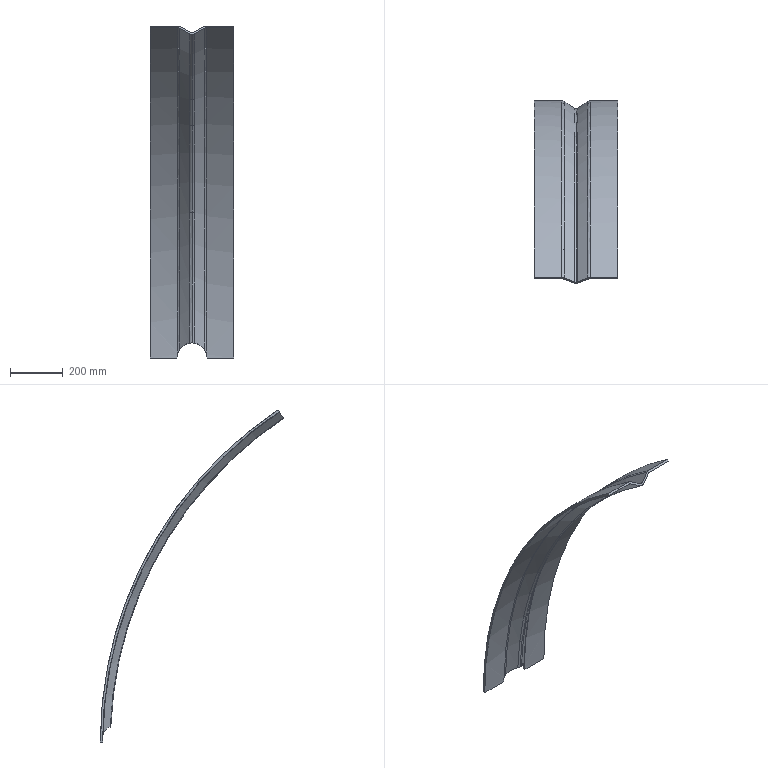Part | SolidWorks | features ICE 1, Sweep 1 | 1 solid | 23 faces | box 317.5 x 695.606 x 1261 mm | volume 3914320 mm3 | torus 8 | cylinder 6 | plane 5 | cone 4 | commonest cylinder face diameters 114.3 x2 3016 x2 3032 x2
STEP:
#1=CARTESIAN_POINT('',(-5.241,-669.592,1237.163));
#2=VERTEX_POINT('',#1);
#3=CARTESIAN_POINT('',(0.,-670.464,1235.856));
#4=VERTEX_POINT('',#3);
#5=CARTESIAN_POINT('',(0.,-665.176,1243.778));
#6=DIRECTION('',(0.,-0.8317,0.5552));
#7=DIRECTION('',(1.,0.,0.));
#8=AXIS2_PLACEMENT_3D('',#5,#6,#7);
#9=CIRCLE('',#8,9.525);
#10=EDGE_CURVE('',#2,#4,#9,.T.);
#11=ORIENTED_EDGE('',*,*,#10,.T.);
#12=CARTESIAN_POINT('',(0.,-10.624,57.15));
#13=VERTEX_POINT('',#12);
#14=CARTESIAN_POINT('',(0.,-1495.425,0.));
#15=DIRECTION('',(-1.,0.,0.));
#16=DIRECTION('',(0.,0.,1.));
#17=AXIS2_PLACEMENT_3D('',#14,#15,#16);
#18=CIRCLE('',#17,1485.9);
#19=EDGE_CURVE('',#4,#13,#18,.T.);
#20=ORIENTED_EDGE('',*,*,#19,.T.);
#21=CARTESIAN_POINT('',(-5.241,-9.042,56.909));
#22=VERTEX_POINT('',#21);
#23=CARTESIAN_POINT('',(-5.241,-9.042,56.909));
#24=CARTESIAN_POINT('',(-4.464,-9.558,56.981));
#25=CARTESIAN_POINT('',(-3.63,-9.95,57.042));
#26=CARTESIAN_POINT('',(-2.518,-10.286,57.095));
#27=CARTESIAN_POINT('',(-2.291,-10.346,57.105));
#28=CARTESIAN_POINT('',(-1.837,-10.447,57.121));
#29=CARTESIAN_POINT('',(-1.609,-10.489,57.128));
#30=CARTESIAN_POINT('',(-0.9231,-10.591,57.144));
#31=CARTESIAN_POINT('',(-0.463,-10.624,57.15));
#32=CARTESIAN_POINT('',(0.,-10.624,57.15));
#33=B_SPLINE_CURVE_WITH_KNOTS('',3,(#23,#24,#25,#26,#27,#28,#29,#30,#31,#32),.UNSPECIFIED.,.F.,.F.,(4,2,2,2,4),(0.000000237,0.002769,0.003461,0.004154,0.005538),.UNSPECIFIED.);
#34=EDGE_CURVE('',#22,#13,#33,.T.);
#35=ORIENTED_EDGE('',*,*,#34,.F.);
#36=CARTESIAN_POINT('',(-5.241,-1495.425,0.));
#37=DIRECTION('',(-1.,0.,0.));
#38=DIRECTION('',(0.,0.,1.));
#39=AXIS2_PLACEMENT_3D('',#36,#37,#38);
#40=CIRCLE('',#39,1487.472);
#41=EDGE_CURVE('',#2,#22,#40,.T.);
#42=ORIENTED_EDGE('',*,*,#41,.F.);
#43=EDGE_LOOP('',(#11,#20,#35,#42));
#44=FACE_OUTER_BOUND('',#43,.T.);
#45=CARTESIAN_POINT('',(0.,-1495.425,0.));
#46=DIRECTION('',(-1.,0.,0.));
#47=DIRECTION('',(0.,0.,1.));
#48=AXIS2_PLACEMENT_3D('',#45,#46,#47);
#49=TOROIDAL_SURFACE('',#48,1495.425,9.525);
#50=ADVANCED_FACE('',(#44),#49,.F.);
#51=CARTESIAN_POINT('',(0.,-674.906,1229.202));
#52=VERTEX_POINT('',#51);
#53=CARTESIAN_POINT('',(9.644,-673.3,1231.607));
#54=VERTEX_POINT('',#53);
#55=CARTESIAN_POINT('',(0.,-665.176,1243.778));
#56=DIRECTION('',(0.,-0.8317,0.5552));
#57=DIRECTION('',(1.,0.,0.));
#58=AXIS2_PLACEMENT_3D('',#55,#56,#57);
#59=CIRCLE('',#58,17.525);
#60=EDGE_CURVE('',#52,#54,#59,.T.);
#61=ORIENTED_EDGE('',*,*,#60,.F.);
#62=CARTESIAN_POINT('',(0.,-18.63,57.15));
#63=VERTEX_POINT('',#62);
#64=CARTESIAN_POINT('',(0.,-1495.425,0.));
#65=DIRECTION('',(-1.,0.,0.));
#66=DIRECTION('',(0.,0.,1.));
#67=AXIS2_PLACEMENT_3D('',#64,#65,#66);
#68=CIRCLE('',#67,1477.9);
#69=EDGE_CURVE('',#52,#63,#68,.T.);
#70=ORIENTED_EDGE('',*,*,#69,.T.);
#71=CARTESIAN_POINT('',(9.644,-15.705,56.33));
#72=VERTEX_POINT('',#71);
#73=CARTESIAN_POINT('',(0.,-18.63,57.15));
#74=CARTESIAN_POINT('',(0.8525,-18.63,57.15));
#75=CARTESIAN_POINT('',(1.717,-18.566,57.13));
#76=CARTESIAN_POINT('',(3.403,-18.314,57.055));
#77=CARTESIAN_POINT('',(4.229,-18.127,56.999));
#78=CARTESIAN_POINT('',(5.447,-17.757,56.891));
#79=CARTESIAN_POINT('',(5.848,-17.619,56.851));
#80=CARTESIAN_POINT('',(6.644,-17.312,56.764));
#81=CARTESIAN_POINT('',(7.038,-17.143,56.716));
#82=CARTESIAN_POINT('',(8.194,-16.596,56.565));
#83=CARTESIAN_POINT('',(8.934,-16.177,56.452));
#84=CARTESIAN_POINT('',(9.644,-15.705,56.33));
#85=B_SPLINE_CURVE_WITH_KNOTS('',3,(#73,#74,#75,#76,#77,#78,#79,#80,#81,#82,#83,#84),.UNSPECIFIED.,.F.,.F.,(4,2,2,2,2,4),(0.01023,0.01277,0.01532,0.0166,0.01787,0.02042),.UNSPECIFIED.);
#86=EDGE_CURVE('',#63,#72,#85,.T.);
#87=ORIENTED_EDGE('',*,*,#86,.T.);
#88=CARTESIAN_POINT('',(9.644,-1495.425,0.));
#89=DIRECTION('',(-1.,0.,0.));
#90=DIRECTION('',(0.,0.,1.));
#91=AXIS2_PLACEMENT_3D('',#88,#89,#90);
#92=CIRCLE('',#91,1480.792);
#93=EDGE_CURVE('',#54,#72,#92,.T.);
#94=ORIENTED_EDGE('',*,*,#93,.F.);
#95=EDGE_LOOP('',(#61,#70,#87,#94));
#96=FACE_OUTER_BOUND('',#95,.T.);
#97=CARTESIAN_POINT('',(0.,-1495.425,0.));
#98=DIRECTION('',(-1.,0.,0.));
#99=DIRECTION('',(0.,0.,1.));
#100=AXIS2_PLACEMENT_3D('',#97,#98,#99);
#101=TOROIDAL_SURFACE('',#100,1495.425,17.525);
#102=ADVANCED_FACE('',(#96),#101,.T.);
#103=ORIENTED_EDGE('',*,*,#86,.F.);
#104=CARTESIAN_POINT('',(0.,-50.,57.15));
#105=DIRECTION('',(0.,1.,0.));
#106=VECTOR('',#105,1000.);
#107=LINE('',#104,#106);
#108=EDGE_CURVE('',#63,#13,#107,.T.);
#109=ORIENTED_EDGE('',*,*,#108,.T.);
#110=CARTESIAN_POINT('',(5.241,-9.042,56.909));
#111=VERTEX_POINT('',#110);
#112=CARTESIAN_POINT('',(0.,-10.624,57.15));
#113=CARTESIAN_POINT('',(0.4615,-10.624,57.15));
#114=CARTESIAN_POINT('',(0.9295,-10.59,57.144));
#115=CARTESIAN_POINT('',(1.845,-10.454,57.122));
#116=CARTESIAN_POINT('',(2.293,-10.354,57.106));
#117=CARTESIAN_POINT('',(3.174,-10.088,57.063));
#118=CARTESIAN_POINT('',(3.608,-9.922,57.038));
#119=CARTESIAN_POINT('',(4.449,-9.527,56.978));
#120=CARTESIAN_POINT('',(4.854,-9.299,56.945));
#121=CARTESIAN_POINT('',(5.241,-9.042,56.909));
#122=B_SPLINE_CURVE_WITH_KNOTS('',3,(#112,#113,#114,#115,#116,#117,#118,#119,#120,#121),.UNSPECIFIED.,.F.,.F.,(4,2,2,2,4),(0.005538,0.006918,0.008298,0.009678,0.01106),.UNSPECIFIED.);
#123=EDGE_CURVE('',#13,#111,#122,.T.);
#124=ORIENTED_EDGE('',*,*,#123,.T.);
#125=CARTESIAN_POINT('',(44.331,17.378,36.067));
#126=VERTEX_POINT('',#125);
#127=CARTESIAN_POINT('',(44.331,17.378,36.067));
#128=CARTESIAN_POINT('',(43.066,16.507,37.622));
#129=CARTESIAN_POINT('',(41.737,15.593,39.09));
#130=CARTESIAN_POINT('',(38.954,13.684,41.864));
#131=CARTESIAN_POINT('',(37.501,12.69,43.169));
#132=CARTESIAN_POINT('',(35.232,11.139,45.008));
#133=CARTESIAN_POINT('',(34.459,10.612,45.603));
#134=CARTESIAN_POINT('',(32.898,9.548,46.741));
#135=CARTESIAN_POINT('',(32.109,9.01,47.287));
#136=CARTESIAN_POINT('',(29.714,7.382,48.855));
#137=CARTESIAN_POINT('',(28.084,6.275,49.809));
#138=CARTESIAN_POINT('',(24.756,4.022,51.544));
#139=CARTESIAN_POINT('',(23.059,2.876,52.325));
#140=CARTESIAN_POINT('',(20.465,1.128,53.368));
#141=CARTESIAN_POINT('',(19.592,0.5412,53.695));
#142=CARTESIAN_POINT('',(17.83,-0.6428,54.305));
#143=CARTESIAN_POINT('',(16.944,-1.238,54.588));
#144=CARTESIAN_POINT('',(12.499,-4.217,55.889));
#145=CARTESIAN_POINT('',(8.895,-6.62,56.573));
#146=CARTESIAN_POINT('',(5.241,-9.042,56.909));
#147=B_SPLINE_CURVE_WITH_KNOTS('',3,(#127,#128,#129,#130,#131,#132,#133,#134,#135,#136,#137,#138,#139,#140,#141,#142,#143,#144,#145,#146),.UNSPECIFIED.,.F.,.F.,(4,2,2,2,2,2,2,2,2,4),(0.007159,0.0137,0.02025,0.02352,0.0268,0.03334,0.03989,0.04316,0.04643,0.05952),.UNSPECIFIED.);
#148=EDGE_CURVE('',#126,#111,#147,.T.);
#149=ORIENTED_EDGE('',*,*,#148,.F.);
#150=CARTESIAN_POINT('',(53.975,20.584,18.784));
#151=VERTEX_POINT('',#150);
#152=CARTESIAN_POINT('',(44.331,17.378,36.067));
#153=CARTESIAN_POINT('',(45.318,18.058,34.854));
#154=CARTESIAN_POINT('',(46.28,18.58,33.57));
#155=CARTESIAN_POINT('',(47.661,19.202,31.547));
#156=CARTESIAN_POINT('',(48.112,19.382,30.856));
#157=CARTESIAN_POINT('',(48.989,19.696,29.442));
#158=CARTESIAN_POINT('',(49.418,19.83,28.718));
#159=CARTESIAN_POINT('',(50.65,20.171,26.523));
#160=CARTESIAN_POINT('',(51.408,20.319,25.023));
#161=CARTESIAN_POINT('',(52.791,20.516,21.955));
#162=CARTESIAN_POINT('',(53.417,20.564,20.386));
#163=CARTESIAN_POINT('',(53.975,20.584,18.784));
#164=B_SPLINE_CURVE_WITH_KNOTS('',3,(#152,#153,#154,#155,#156,#157,#158,#159,#160,#161,#162,#163),.UNSPECIFIED.,.F.,.F.,(4,2,2,2,2,4),(0.000000341,0.005054,0.007581,0.01011,0.01516,0.02022),.UNSPECIFIED.);
#165=EDGE_CURVE('',#126,#151,#164,.T.);
#166=ORIENTED_EDGE('',*,*,#165,.T.);
#167=CARTESIAN_POINT('',(57.15,20.7,0.));
#168=VERTEX_POINT('',#167);
#169=CARTESIAN_POINT('',(57.15,20.7,0.));
#170=CARTESIAN_POINT('',(57.15,20.7,3.22));
#171=CARTESIAN_POINT('',(56.88,20.69,6.395));
#172=CARTESIAN_POINT('',(55.821,20.65,12.656));
#173=CARTESIAN_POINT('',(55.033,20.621,15.743));
#174=CARTESIAN_POINT('',(53.975,20.584,18.784));
#175=B_SPLINE_CURVE_WITH_KNOTS('',3,(#169,#170,#171,#172,#173,#174),.UNSPECIFIED.,.F.,.F.,(4,2,4),(0.,0.009525,0.01905),.UNSPECIFIED.);
#176=EDGE_CURVE('',#168,#151,#175,.T.);
#177=ORIENTED_EDGE('',*,*,#176,.F.);
#178=CARTESIAN_POINT('',(57.15,12.7,0.));
#179=VERTEX_POINT('',#178);
#180=CARTESIAN_POINT('',(57.15,-50.,0.));
#181=DIRECTION('',(0.,1.,0.));
#182=VECTOR('',#181,1000.);
#183=LINE('',#180,#182);
#184=EDGE_CURVE('',#179,#168,#183,.T.);
#185=ORIENTED_EDGE('',*,*,#184,.F.);
#186=CARTESIAN_POINT('',(53.975,12.583,18.784));
#187=VERTEX_POINT('',#186);
#188=CARTESIAN_POINT('',(57.15,12.7,0.));
#189=CARTESIAN_POINT('',(57.15,12.7,3.22));
#190=CARTESIAN_POINT('',(56.88,12.69,6.395));
#191=CARTESIAN_POINT('',(55.821,12.65,12.656));
#192=CARTESIAN_POINT('',(55.033,12.621,15.743));
#193=CARTESIAN_POINT('',(53.975,12.583,18.784));
#194=B_SPLINE_CURVE_WITH_KNOTS('',3,(#188,#189,#190,#191,#192,#193),.UNSPECIFIED.,.F.,.F.,(4,2,4),(0.,0.009525,0.01905),.UNSPECIFIED.);
#195=EDGE_CURVE('',#179,#187,#194,.T.);
#196=ORIENTED_EDGE('',*,*,#195,.T.);
#197=CARTESIAN_POINT('',(48.734,10.832,29.852));
#198=VERTEX_POINT('',#197);
#199=CARTESIAN_POINT('',(48.734,10.832,29.852));
#200=CARTESIAN_POINT('',(49.248,11.188,29.013));
#201=CARTESIAN_POINT('',(49.748,11.464,28.148));
#202=CARTESIAN_POINT('',(50.71,11.908,26.375));
#203=CARTESIAN_POINT('',(51.172,12.075,25.467));
#204=CARTESIAN_POINT('',(52.055,12.331,23.611));
#205=CARTESIAN_POINT('',(52.476,12.42,22.66));
#206=CARTESIAN_POINT('',(53.264,12.539,20.739));
#207=CARTESIAN_POINT('',(53.633,12.571,19.767));
#208=CARTESIAN_POINT('',(53.975,12.583,18.784));
#209=B_SPLINE_CURVE_WITH_KNOTS('',3,(#199,#200,#201,#202,#203,#204,#205,#206,#207,#208),.UNSPECIFIED.,.F.,.F.,(4,2,2,2,4),(0.000000402,0.003097,0.006194,0.009291,0.01239),.UNSPECIFIED.);
#210=EDGE_CURVE('',#198,#187,#209,.T.);
#211=ORIENTED_EDGE('',*,*,#210,.F.);
#212=CARTESIAN_POINT('',(48.734,10.832,29.852));
#213=CARTESIAN_POINT('',(47.603,10.051,31.698));
#214=CARTESIAN_POINT('',(46.381,9.207,33.459));
#215=CARTESIAN_POINT('',(44.417,7.853,35.978));
#216=CARTESIAN_POINT('',(43.74,7.387,36.797));
#217=CARTESIAN_POINT('',(42.344,6.427,38.396));
#218=CARTESIAN_POINT('',(41.625,5.933,39.173));
#219=CARTESIAN_POINT('',(39.431,4.427,41.421));
#220=CARTESIAN_POINT('',(37.91,3.384,42.815));
#221=CARTESIAN_POINT('',(34.757,1.229,45.412));
#222=CARTESIAN_POINT('',(33.126,0.1169,46.614));
#223=CARTESIAN_POINT('',(29.759,-2.174,48.832));
#224=CARTESIAN_POINT('',(28.016,-3.358,49.852));
#225=CARTESIAN_POINT('',(24.486,-5.747,51.677));
#226=CARTESIAN_POINT('',(22.694,-6.958,52.488));
#227=CARTESIAN_POINT('',(19.055,-9.408,53.915));
#228=CARTESIAN_POINT('',(17.21,-10.648,54.532));
#229=CARTESIAN_POINT('',(14.401,-12.529,55.314));
#230=CARTESIAN_POINT('',(13.459,-13.159,55.551));
#231=CARTESIAN_POINT('',(11.56,-14.427,55.977));
#232=CARTESIAN_POINT('',(10.603,-15.066,56.166));
#233=CARTESIAN_POINT('',(9.644,-15.705,56.33));
#234=B_SPLINE_CURVE_WITH_KNOTS('',3,(#212,#213,#214,#215,#216,#217,#218,#219,#220,#221,#222,#223,#224,#225,#226,#227,#228,#229,#230,#231,#232,#233),.UNSPECIFIED.,.F.,.F.,(4,2,2,2,2,2,2,2,2,2,4),(0.008928,0.01583,0.01928,0.02273,0.02964,0.03654,0.04344,0.05035,0.05725,0.0607,0.06415),.UNSPECIFIED.);
#235=EDGE_CURVE('',#198,#72,#234,.T.);
#236=ORIENTED_EDGE('',*,*,#235,.T.);
#237=EDGE_LOOP('',(#103,#109,#124,#149,#166,#177,#185,#196,#211,#236));
#238=FACE_OUTER_BOUND('',#237,.T.);
#239=CARTESIAN_POINT('',(0.,-50.,0.));
#240=DIRECTION('',(0.,1.,0.));
#241=DIRECTION('',(0.,0.,1.));
#242=AXIS2_PLACEMENT_3D('',#239,#240,#241);
#243=CYLINDRICAL_SURFACE('',#242,57.15);
#244=ADVANCED_FACE('',(#238),#243,.F.);
#245=CARTESIAN_POINT('',(158.75,12.7,0.));
#246=VERTEX_POINT('',#245);
#247=CARTESIAN_POINT('',(158.75,12.7,0.));
#248=DIRECTION('',(-1.,0.,0.));
#249=VECTOR('',#248,1000.);
#250=LINE('',#247,#249);
#251=EDGE_CURVE('',#246,#179,#250,.T.);
#252=ORIENTED_EDGE('',*,*,#251,.T.);
#253=ORIENTED_EDGE('',*,*,#184,.T.);
#254=CARTESIAN_POINT('',(158.75,20.7,0.));
#255=VERTEX_POINT('',#254);
#256=CARTESIAN_POINT('',(158.75,20.7,0.));
#257=DIRECTION('',(-1.,0.,0.));
#258=VECTOR('',#257,1000.);
#259=LINE('',#256,#258);
#260=EDGE_CURVE('',#255,#168,#259,.T.);
#261=ORIENTED_EDGE('',*,*,#260,.F.);
#262=CARTESIAN_POINT('',(158.75,20.7,0.));
#263=DIRECTION('',(0.,-1.,0.));
#264=VECTOR('',#263,1000.);
#265=LINE('',#262,#264);
#266=EDGE_CURVE('',#255,#246,#265,.T.);
#267=ORIENTED_EDGE('',*,*,#266,.T.);
#268=EDGE_LOOP('',(#252,#253,#261,#267));
#269=FACE_OUTER_BOUND('',#268,.T.);
#270=CARTESIAN_POINT('',(-53.975,3.175,0.));
#271=DIRECTION('',(0.,0.,1.));
#272=DIRECTION('',(1.,0.,0.));
#273=AXIS2_PLACEMENT_3D('',#270,#271,#272);
#274=PLANE('',#273);
#275=ADVANCED_FACE('',(#269),#274,.F.);
#276=CARTESIAN_POINT('',(-158.75,-658.125,1254.341));
#277=VERTEX_POINT('',#276);
#278=CARTESIAN_POINT('',(-158.75,12.7,0.));
#279=VERTEX_POINT('',#278);
#280=CARTESIAN_POINT('',(-158.75,-1495.425,0.));
#281=DIRECTION('',(-1.,0.,0.));
#282=DIRECTION('',(0.,0.,1.));
#283=AXIS2_PLACEMENT_3D('',#280,#281,#282);
#284=CIRCLE('',#283,1508.125);
#285=EDGE_CURVE('',#277,#279,#284,.T.);
#286=ORIENTED_EDGE('',*,*,#285,.F.);
#287=CARTESIAN_POINT('',(-158.75,-653.684,1260.994));
#288=VERTEX_POINT('',#287);
#289=CARTESIAN_POINT('',(-158.75,-653.684,1260.994));
#290=DIRECTION('',(0.,-0.5552,-0.8317));
#291=VECTOR('',#290,1000.);
#292=LINE('',#289,#291);
#293=EDGE_CURVE('',#288,#277,#292,.T.);
#294=ORIENTED_EDGE('',*,*,#293,.F.);
#295=CARTESIAN_POINT('',(-158.75,20.7,0.));
#296=VERTEX_POINT('',#295);
#297=CARTESIAN_POINT('',(-158.75,-1495.425,0.));
#298=DIRECTION('',(-1.,0.,0.));
#299=DIRECTION('',(0.,0.,1.));
#300=AXIS2_PLACEMENT_3D('',#297,#298,#299);
#301=CIRCLE('',#300,1516.125);
#302=EDGE_CURVE('',#288,#296,#301,.T.);
#303=ORIENTED_EDGE('',*,*,#302,.T.);
#304=CARTESIAN_POINT('',(-158.75,20.7,0.));
#305=DIRECTION('',(0.,-1.,0.));
#306=VECTOR('',#305,1000.);
#307=LINE('',#304,#306);
#308=EDGE_CURVE('',#296,#279,#307,.T.);
#309=ORIENTED_EDGE('',*,*,#308,.T.);
#310=EDGE_LOOP('',(#286,#294,#303,#309));
#311=FACE_OUTER_BOUND('',#310,.T.);
#312=CARTESIAN_POINT('',(-158.75,-653.684,1260.994));
#313=DIRECTION('',(1.,0.,0.));
#314=DIRECTION('',(0.,0.,-1.));
#315=AXIS2_PLACEMENT_3D('',#312,#313,#314);
#316=PLANE('',#315);
#317=ADVANCED_FACE('',(#311),#316,.F.);
#318=CARTESIAN_POINT('',(-57.15,12.7,0.));
#319=VERTEX_POINT('',#318);
#320=CARTESIAN_POINT('',(-158.75,12.7,0.));
#321=DIRECTION('',(1.,0.,0.));
#322=VECTOR('',#321,1000.);
#323=LINE('',#320,#322);
#324=EDGE_CURVE('',#279,#319,#323,.T.);
#325=ORIENTED_EDGE('',*,*,#324,.T.);
#326=CARTESIAN_POINT('',(-53.975,12.583,18.784));
#327=VERTEX_POINT('',#326);
#328=CARTESIAN_POINT('',(-57.15,12.7,0.));
#329=CARTESIAN_POINT('',(-57.15,12.7,3.22));
#330=CARTESIAN_POINT('',(-56.88,12.69,6.395));
#331=CARTESIAN_POINT('',(-55.821,12.65,12.656));
#332=CARTESIAN_POINT('',(-55.033,12.621,15.743));
#333=CARTESIAN_POINT('',(-53.975,12.583,18.784));
#334=B_SPLINE_CURVE_WITH_KNOTS('',3,(#328,#329,#330,#331,#332,#333),.UNSPECIFIED.,.F.,.F.,(4,2,4),(0.,0.009525,0.01905),.UNSPECIFIED.);
#335=EDGE_CURVE('',#319,#327,#334,.T.);
#336=ORIENTED_EDGE('',*,*,#335,.T.);
#337=CARTESIAN_POINT('',(-53.975,-658.125,1254.341));
#338=VERTEX_POINT('',#337);
#339=CARTESIAN_POINT('',(-53.975,-1495.425,0.));
#340=DIRECTION('',(-1.,0.,0.));
#341=DIRECTION('',(0.,0.,1.));
#342=AXIS2_PLACEMENT_3D('',#339,#340,#341);
#343=CIRCLE('',#342,1508.125);
#344=EDGE_CURVE('',#338,#327,#343,.T.);
#345=ORIENTED_EDGE('',*,*,#344,.F.);
#346=CARTESIAN_POINT('',(-158.75,-658.125,1254.341));
#347=DIRECTION('',(1.,0.,0.));
#348=VECTOR('',#347,1000.);
#349=LINE('',#346,#348);
#350=EDGE_CURVE('',#277,#338,#349,.T.);
#351=ORIENTED_EDGE('',*,*,#350,.F.);
#352=ORIENTED_EDGE('',*,*,#285,.T.);
#353=EDGE_LOOP('',(#325,#336,#345,#351,#352));
#354=FACE_OUTER_BOUND('',#353,.T.);
#355=CARTESIAN_POINT('',(0.,-1495.425,0.));
#356=DIRECTION('',(-1.,0.,0.));
#357=DIRECTION('',(0.,0.,1.));
#358=AXIS2_PLACEMENT_3D('',#355,#356,#357);
#359=CYLINDRICAL_SURFACE('',#358,1508.125);
#360=ADVANCED_FACE('',(#354),#359,.F.);
#361=CARTESIAN_POINT('',(-48.734,10.832,29.852));
#362=VERTEX_POINT('',#361);
#363=CARTESIAN_POINT('',(-48.734,10.832,29.852));
#364=CARTESIAN_POINT('',(-49.248,11.188,29.013));
#365=CARTESIAN_POINT('',(-49.748,11.464,28.148));
#366=CARTESIAN_POINT('',(-50.71,11.908,26.375));
#367=CARTESIAN_POINT('',(-51.172,12.075,25.467));
#368=CARTESIAN_POINT('',(-52.055,12.331,23.611));
#369=CARTESIAN_POINT('',(-52.476,12.42,22.66));
#370=CARTESIAN_POINT('',(-53.264,12.539,20.739));
#371=CARTESIAN_POINT('',(-53.633,12.571,19.767));
#372=CARTESIAN_POINT('',(-53.975,12.583,18.784));
#373=B_SPLINE_CURVE_WITH_KNOTS('',3,(#363,#364,#365,#366,#367,#368,#369,#370,#371,#372),.UNSPECIFIED.,.F.,.F.,(4,2,2,2,4),(0.000000402,0.003097,0.006194,0.009291,0.01239),.UNSPECIFIED.);
#374=EDGE_CURVE('',#362,#327,#373,.T.);
#375=ORIENTED_EDGE('',*,*,#374,.F.);
#376=CARTESIAN_POINT('',(-48.734,-658.998,1253.033));
#377=VERTEX_POINT('',#376);
#378=CARTESIAN_POINT('',(-48.734,-1495.425,0.));
#379=DIRECTION('',(-1.,0.,0.));
#380=DIRECTION('',(0.,0.,1.));
#381=AXIS2_PLACEMENT_3D('',#378,#379,#380);
#382=CIRCLE('',#381,1506.553);
#383=EDGE_CURVE('',#377,#362,#382,.T.);
#384=ORIENTED_EDGE('',*,*,#383,.F.);
#385=CARTESIAN_POINT('',(-53.975,-663.413,1246.418));
#386=DIRECTION('',(0.,-0.8317,0.5552));
#387=DIRECTION('',(1.,0.,0.));
#388=AXIS2_PLACEMENT_3D('',#385,#386,#387);
#389=CIRCLE('',#388,9.525);
#390=EDGE_CURVE('',#377,#338,#389,.T.);
#391=ORIENTED_EDGE('',*,*,#390,.T.);
#392=ORIENTED_EDGE('',*,*,#344,.T.);
#393=EDGE_LOOP('',(#375,#384,#391,#392));
#394=FACE_OUTER_BOUND('',#393,.T.);
#395=CARTESIAN_POINT('',(-53.975,-1495.425,0.));
#396=DIRECTION('',(-1.,0.,0.));
#397=DIRECTION('',(0.,0.,1.));
#398=AXIS2_PLACEMENT_3D('',#395,#396,#397);
#399=TOROIDAL_SURFACE('',#398,1498.6,9.525);
#400=ADVANCED_FACE('',(#394),#399,.F.);
#401=ORIENTED_EDGE('',*,*,#383,.T.);
#402=CARTESIAN_POINT('',(-9.644,-15.705,56.33));
#403=VERTEX_POINT('',#402);
#404=CARTESIAN_POINT('',(-48.734,10.832,29.852));
#405=CARTESIAN_POINT('',(-47.603,10.051,31.698));
#406=CARTESIAN_POINT('',(-46.381,9.207,33.459));
#407=CARTESIAN_POINT('',(-44.417,7.853,35.978));
#408=CARTESIAN_POINT('',(-43.74,7.387,36.797));
#409=CARTESIAN_POINT('',(-42.344,6.427,38.396));
#410=CARTESIAN_POINT('',(-41.625,5.933,39.173));
#411=CARTESIAN_POINT('',(-39.431,4.427,41.421));
#412=CARTESIAN_POINT('',(-37.91,3.384,42.815));
#413=CARTESIAN_POINT('',(-34.757,1.229,45.412));
#414=CARTESIAN_POINT('',(-33.126,0.1169,46.614));
#415=CARTESIAN_POINT('',(-29.759,-2.174,48.832));
#416=CARTESIAN_POINT('',(-28.016,-3.358,49.852));
#417=CARTESIAN_POINT('',(-24.486,-5.747,51.677));
#418=CARTESIAN_POINT('',(-22.694,-6.958,52.488));
#419=CARTESIAN_POINT('',(-19.055,-9.408,53.915));
#420=CARTESIAN_POINT('',(-17.21,-10.648,54.532));
#421=CARTESIAN_POINT('',(-14.401,-12.529,55.314));
#422=CARTESIAN_POINT('',(-13.459,-13.159,55.551));
#423=CARTESIAN_POINT('',(-11.56,-14.427,55.977));
#424=CARTESIAN_POINT('',(-10.603,-15.066,56.166));
#425=CARTESIAN_POINT('',(-9.644,-15.705,56.33));
#426=B_SPLINE_CURVE_WITH_KNOTS('',3,(#404,#405,#406,#407,#408,#409,#410,#411,#412,#413,#414,#415,#416,#417,#418,#419,#420,#421,#422,#423,#424,#425),.UNSPECIFIED.,.F.,.F.,(4,2,2,2,2,2,2,2,2,2,4),(0.008928,0.01583,0.01928,0.02273,0.02964,0.03654,0.04344,0.05035,0.05725,0.0607,0.06415),.UNSPECIFIED.);
#427=EDGE_CURVE('',#362,#403,#426,.T.);
#428=ORIENTED_EDGE('',*,*,#427,.T.);
#429=CARTESIAN_POINT('',(-9.644,-673.3,1231.607));
#430=VERTEX_POINT('',#429);
#431=CARTESIAN_POINT('',(-9.644,-1495.425,0.));
#432=DIRECTION('',(-1.,0.,0.));
#433=DIRECTION('',(0.,0.,1.));
#434=AXIS2_PLACEMENT_3D('',#431,#432,#433);
#435=CIRCLE('',#434,1480.792);
#436=EDGE_CURVE('',#430,#403,#435,.T.);
#437=ORIENTED_EDGE('',*,*,#436,.F.);
#438=CARTESIAN_POINT('',(-48.734,-658.998,1253.033));
#439=DIRECTION('',(0.835,-0.3055,-0.4577));
#440=VECTOR('',#439,1000.);
#441=LINE('',#438,#440);
#442=EDGE_CURVE('',#377,#430,#441,.T.);
#443=ORIENTED_EDGE('',*,*,#442,.F.);
#444=EDGE_LOOP('',(#401,#428,#437,#443));
#445=FACE_OUTER_BOUND('',#444,.T.);
#446=CARTESIAN_POINT('',(-48.734,-1495.425,0.));
#447=DIRECTION('',(-1.,0.,0.));
#448=DIRECTION('',(0.,0.,1.));
#449=AXIS2_PLACEMENT_3D('',#446,#447,#448);
#450=CONICAL_SURFACE('',#449,1506.553,0.5827);
#451=ADVANCED_FACE('',(#445),#450,.F.);
#452=ORIENTED_EDGE('',*,*,#69,.F.);
#453=CARTESIAN_POINT('',(0.,-665.176,1243.778));
#454=DIRECTION('',(0.,-0.8317,0.5552));
#455=DIRECTION('',(1.,0.,0.));
#456=AXIS2_PLACEMENT_3D('',#453,#454,#455);
#457=CIRCLE('',#456,17.525);
#458=EDGE_CURVE('',#430,#52,#457,.T.);
#459=ORIENTED_EDGE('',*,*,#458,.F.);
#460=ORIENTED_EDGE('',*,*,#436,.T.);
#461=CARTESIAN_POINT('',(-9.644,-15.705,56.33));
#462=CARTESIAN_POINT('',(-8.932,-16.179,56.452));
#463=CARTESIAN_POINT('',(-8.193,-16.596,56.565));
#464=CARTESIAN_POINT('',(-6.663,-17.321,56.766));
#465=CARTESIAN_POINT('',(-5.872,-17.628,56.854));
#466=CARTESIAN_POINT('',(-4.643,-18.002,56.963));
#467=CARTESIAN_POINT('',(-4.225,-18.113,56.995));
#468=CARTESIAN_POINT('',(-3.388,-18.301,57.051));
#469=CARTESIAN_POINT('',(-2.969,-18.379,57.074));
#470=CARTESIAN_POINT('',(-1.705,-18.567,57.131));
#471=CARTESIAN_POINT('',(-0.8555,-18.63,57.15));
#472=CARTESIAN_POINT('',(0.,-18.63,57.15));
#473=B_SPLINE_CURVE_WITH_KNOTS('',3,(#461,#462,#463,#464,#465,#466,#467,#468,#469,#470,#471,#472),.UNSPECIFIED.,.F.,.F.,(4,2,2,2,2,4),(0.000000239,0.002557,0.005113,0.006392,0.00767,0.01023),.UNSPECIFIED.);
#474=EDGE_CURVE('',#403,#63,#473,.T.);
#475=ORIENTED_EDGE('',*,*,#474,.T.);
#476=EDGE_LOOP('',(#452,#459,#460,#475));
#477=FACE_OUTER_BOUND('',#476,.T.);
#478=CARTESIAN_POINT('',(0.,-1495.425,0.));
#479=DIRECTION('',(-1.,0.,0.));
#480=DIRECTION('',(0.,0.,1.));
#481=AXIS2_PLACEMENT_3D('',#478,#479,#480);
#482=TOROIDAL_SURFACE('',#481,1495.425,17.525);
#483=ADVANCED_FACE('',(#477),#482,.T.);
#484=ORIENTED_EDGE('',*,*,#235,.F.);
#485=CARTESIAN_POINT('',(48.734,-658.998,1253.033));
#486=VERTEX_POINT('',#485);
#487=CARTESIAN_POINT('',(48.734,-1495.425,0.));
#488=DIRECTION('',(-1.,0.,0.));
#489=DIRECTION('',(0.,0.,1.));
#490=AXIS2_PLACEMENT_3D('',#487,#488,#489);
#491=CIRCLE('',#490,1506.553);
#492=EDGE_CURVE('',#486,#198,#491,.T.);
#493=ORIENTED_EDGE('',*,*,#492,.F.);
#494=CARTESIAN_POINT('',(48.734,-658.998,1253.033));
#495=DIRECTION('',(-0.835,-0.3055,-0.4577));
#496=VECTOR('',#495,1000.);
#497=LINE('',#494,#496);
#498=EDGE_CURVE('',#486,#54,#497,.T.);
#499=ORIENTED_EDGE('',*,*,#498,.T.);
#500=ORIENTED_EDGE('',*,*,#93,.T.);
#501=EDGE_LOOP('',(#484,#493,#499,#500));
#502=FACE_OUTER_BOUND('',#501,.T.);
#503=CARTESIAN_POINT('',(48.734,-1495.425,0.));
#504=DIRECTION('',(1.,0.,0.));
#505=DIRECTION('',(0.,0.,-1.));
#506=AXIS2_PLACEMENT_3D('',#503,#504,#505);
#507=CONICAL_SURFACE('',#506,1506.553,0.5827);
#508=ADVANCED_FACE('',(#502),#507,.F.);
#509=ORIENTED_EDGE('',*,*,#492,.T.);
#510=ORIENTED_EDGE('',*,*,#210,.T.);
#511=CARTESIAN_POINT('',(53.975,-658.125,1254.341));
#512=VERTEX_POINT('',#511);
#513=CARTESIAN_POINT('',(53.975,-1495.425,0.));
#514=DIRECTION('',(-1.,0.,0.));
#515=DIRECTION('',(0.,0.,1.));
#516=AXIS2_PLACEMENT_3D('',#513,#514,#515);
#517=CIRCLE('',#516,1508.125);
#518=EDGE_CURVE('',#512,#187,#517,.T.);
#519=ORIENTED_EDGE('',*,*,#518,.F.);
#520=CARTESIAN_POINT('',(53.975,-663.413,1246.418));
#521=DIRECTION('',(0.,0.8317,-0.5552));
#522=DIRECTION('',(-1.,0.,0.));
#523=AXIS2_PLACEMENT_3D('',#520,#521,#522);
#524=CIRCLE('',#523,9.525);
#525=EDGE_CURVE('',#486,#512,#524,.T.);
#526=ORIENTED_EDGE('',*,*,#525,.F.);
#527=EDGE_LOOP('',(#509,#510,#519,#526));
#528=FACE_OUTER_BOUND('',#527,.T.);
#529=CARTESIAN_POINT('',(53.975,-1495.425,0.));
#530=DIRECTION('',(-1.,0.,0.));
#531=DIRECTION('',(0.,0.,1.));
#532=AXIS2_PLACEMENT_3D('',#529,#530,#531);
#533=TOROIDAL_SURFACE('',#532,1498.6,9.525);
#534=ADVANCED_FACE('',(#528),#533,.F.);
#535=ORIENTED_EDGE('',*,*,#195,.F.);
#536=ORIENTED_EDGE('',*,*,#251,.F.);
#537=CARTESIAN_POINT('',(158.75,-658.125,1254.341));
#538=VERTEX_POINT('',#537);
#539=CARTESIAN_POINT('',(158.75,-1495.425,0.));
#540=DIRECTION('',(-1.,0.,0.));
#541=DIRECTION('',(0.,0.,1.));
#542=AXIS2_PLACEMENT_3D('',#539,#540,#541);
#543=CIRCLE('',#542,1508.125);
#544=EDGE_CURVE('',#538,#246,#543,.T.);
#545=ORIENTED_EDGE('',*,*,#544,.F.);
#546=CARTESIAN_POINT('',(158.75,-658.125,1254.341));
#547=DIRECTION('',(-1.,0.,0.));
#548=VECTOR('',#547,1000.);
#549=LINE('',#546,#548);
#550=EDGE_CURVE('',#538,#512,#549,.T.);
#551=ORIENTED_EDGE('',*,*,#550,.T.);
#552=ORIENTED_EDGE('',*,*,#518,.T.);
#553=EDGE_LOOP('',(#535,#536,#545,#551,#552));
#554=FACE_OUTER_BOUND('',#553,.T.);
#555=CARTESIAN_POINT('',(0.,-1495.425,0.));
#556=DIRECTION('',(-1.,0.,0.));
#557=DIRECTION('',(0.,0.,1.));
#558=AXIS2_PLACEMENT_3D('',#555,#556,#557);
#559=CYLINDRICAL_SURFACE('',#558,1508.125);
#560=ADVANCED_FACE('',(#554),#559,.F.);
#561=CARTESIAN_POINT('',(158.75,-653.684,1260.994));
#562=VERTEX_POINT('',#561);
#563=CARTESIAN_POINT('',(158.75,-1495.425,0.));
#564=DIRECTION('',(-1.,0.,0.));
#565=DIRECTION('',(0.,0.,1.));
#566=AXIS2_PLACEMENT_3D('',#563,#564,#565);
#567=CIRCLE('',#566,1516.125);
#568=EDGE_CURVE('',#562,#255,#567,.T.);
#569=ORIENTED_EDGE('',*,*,#568,.F.);
#570=CARTESIAN_POINT('',(158.75,-653.684,1260.994));
#571=DIRECTION('',(0.,-0.5552,-0.8317));
#572=VECTOR('',#571,1000.);
#573=LINE('',#570,#572);
#574=EDGE_CURVE('',#562,#538,#573,.T.);
#575=ORIENTED_EDGE('',*,*,#574,.T.);
#576=ORIENTED_EDGE('',*,*,#544,.T.);
#577=ORIENTED_EDGE('',*,*,#266,.F.);
#578=EDGE_LOOP('',(#569,#575,#576,#577));
#579=FACE_OUTER_BOUND('',#578,.T.);
#580=CARTESIAN_POINT('',(158.75,-653.684,1260.994));
#581=DIRECTION('',(1.,0.,0.));
#582=DIRECTION('',(0.,0.,-1.));
#583=AXIS2_PLACEMENT_3D('',#580,#581,#582);
#584=PLANE('',#583);
#585=ADVANCED_FACE('',(#579),#584,.T.);
#586=ORIENTED_EDGE('',*,*,#260,.T.);
#587=ORIENTED_EDGE('',*,*,#176,.T.);
#588=CARTESIAN_POINT('',(53.975,-653.684,1260.994));
#589=VERTEX_POINT('',#588);
#590=CARTESIAN_POINT('',(53.975,-1495.425,0.));
#591=DIRECTION('',(-1.,0.,0.));
#592=DIRECTION('',(0.,0.,1.));
#593=AXIS2_PLACEMENT_3D('',#590,#591,#592);
#594=CIRCLE('',#593,1516.125);
#595=EDGE_CURVE('',#589,#151,#594,.T.);
#596=ORIENTED_EDGE('',*,*,#595,.F.);
#597=CARTESIAN_POINT('',(158.75,-653.684,1260.994));
#598=DIRECTION('',(-1.,0.,0.));
#599=VECTOR('',#598,1000.);
#600=LINE('',#597,#599);
#601=EDGE_CURVE('',#562,#589,#600,.T.);
#602=ORIENTED_EDGE('',*,*,#601,.F.);
#603=ORIENTED_EDGE('',*,*,#568,.T.);
#604=EDGE_LOOP('',(#586,#587,#596,#602,#603));
#605=FACE_OUTER_BOUND('',#604,.T.);
#606=CARTESIAN_POINT('',(0.,-1495.425,0.));
#607=DIRECTION('',(-1.,0.,0.));
#608=DIRECTION('',(0.,0.,1.));
#609=AXIS2_PLACEMENT_3D('',#606,#607,#608);
#610=CYLINDRICAL_SURFACE('',#609,1516.125);
#611=ADVANCED_FACE('',(#605),#610,.T.);
#612=ORIENTED_EDGE('',*,*,#165,.F.);
#613=CARTESIAN_POINT('',(44.331,-655.289,1258.589));
#614=VERTEX_POINT('',#613);
#615=CARTESIAN_POINT('',(44.331,-1495.425,0.));
#616=DIRECTION('',(-1.,0.,0.));
#617=DIRECTION('',(0.,0.,1.));
#618=AXIS2_PLACEMENT_3D('',#615,#616,#617);
#619=CIRCLE('',#618,1513.233);
#620=EDGE_CURVE('',#614,#126,#619,.T.);
#621=ORIENTED_EDGE('',*,*,#620,.F.);
#622=CARTESIAN_POINT('',(53.975,-663.413,1246.418));
#623=DIRECTION('',(0.,0.8317,-0.5552));
#624=DIRECTION('',(-1.,0.,0.));
#625=AXIS2_PLACEMENT_3D('',#622,#623,#624);
#626=CIRCLE('',#625,17.525);
#627=EDGE_CURVE('',#614,#589,#626,.T.);
#628=ORIENTED_EDGE('',*,*,#627,.T.);
#629=ORIENTED_EDGE('',*,*,#595,.T.);
#630=EDGE_LOOP('',(#612,#621,#628,#629));
#631=FACE_OUTER_BOUND('',#630,.T.);
#632=CARTESIAN_POINT('',(53.975,-1495.425,0.));
#633=DIRECTION('',(-1.,0.,0.));
#634=DIRECTION('',(0.,0.,1.));
#635=AXIS2_PLACEMENT_3D('',#632,#633,#634);
#636=TOROIDAL_SURFACE('',#635,1498.6,17.525);
#637=ADVANCED_FACE('',(#631),#636,.T.);
#638=ORIENTED_EDGE('',*,*,#620,.T.);
#639=ORIENTED_EDGE('',*,*,#148,.T.);
#640=CARTESIAN_POINT('',(5.241,-669.592,1237.163));
#641=VERTEX_POINT('',#640);
#642=CARTESIAN_POINT('',(5.241,-1495.425,0.));
#643=DIRECTION('',(-1.,0.,0.));
#644=DIRECTION('',(0.,0.,1.));
#645=AXIS2_PLACEMENT_3D('',#642,#643,#644);
#646=CIRCLE('',#645,1487.472);
#647=EDGE_CURVE('',#641,#111,#646,.T.);
#648=ORIENTED_EDGE('',*,*,#647,.F.);
#649=CARTESIAN_POINT('',(44.331,-655.289,1258.589));
#650=DIRECTION('',(-0.835,-0.3055,-0.4577));
#651=VECTOR('',#650,1000.);
#652=LINE('',#649,#651);
#653=EDGE_CURVE('',#614,#641,#652,.T.);
#654=ORIENTED_EDGE('',*,*,#653,.F.);
#655=EDGE_LOOP('',(#638,#639,#648,#654));
#656=FACE_OUTER_BOUND('',#655,.T.);
#657=CARTESIAN_POINT('',(44.331,-1495.425,0.));
#658=DIRECTION('',(1.,0.,0.));
#659=DIRECTION('',(0.,0.,-1.));
#660=AXIS2_PLACEMENT_3D('',#657,#658,#659);
#661=CONICAL_SURFACE('',#660,1513.233,0.5827);
#662=ADVANCED_FACE('',(#656),#661,.T.);
#663=ORIENTED_EDGE('',*,*,#19,.F.);
#664=CARTESIAN_POINT('',(0.,-665.176,1243.778));
#665=DIRECTION('',(0.,-0.8317,0.5552));
#666=DIRECTION('',(1.,0.,0.));
#667=AXIS2_PLACEMENT_3D('',#664,#665,#666);
#668=CIRCLE('',#667,9.525);
#669=EDGE_CURVE('',#4,#641,#668,.T.);
#670=ORIENTED_EDGE('',*,*,#669,.T.);
#671=ORIENTED_EDGE('',*,*,#647,.T.);
#672=ORIENTED_EDGE('',*,*,#123,.F.);
#673=EDGE_LOOP('',(#663,#670,#671,#672));
#674=FACE_OUTER_BOUND('',#673,.T.);
#675=CARTESIAN_POINT('',(0.,-1495.425,0.));
#676=DIRECTION('',(-1.,0.,0.));
#677=DIRECTION('',(0.,0.,1.));
#678=AXIS2_PLACEMENT_3D('',#675,#676,#677);
#679=TOROIDAL_SURFACE('',#678,1495.425,9.525);
#680=ADVANCED_FACE('',(#674),#679,.F.);
#681=CARTESIAN_POINT('',(-44.331,17.378,36.067));
#682=VERTEX_POINT('',#681);
#683=CARTESIAN_POINT('',(-44.331,17.378,36.067));
#684=CARTESIAN_POINT('',(-43.066,16.507,37.622));
#685=CARTESIAN_POINT('',(-41.737,15.593,39.09));
#686=CARTESIAN_POINT('',(-38.954,13.684,41.864));
#687=CARTESIAN_POINT('',(-37.501,12.69,43.169));
#688=CARTESIAN_POINT('',(-35.232,11.139,45.008));
#689=CARTESIAN_POINT('',(-34.459,10.612,45.603));
#690=CARTESIAN_POINT('',(-32.898,9.548,46.741));
#691=CARTESIAN_POINT('',(-32.109,9.01,47.287));
#692=CARTESIAN_POINT('',(-29.714,7.382,48.855));
#693=CARTESIAN_POINT('',(-28.084,6.275,49.809));
#694=CARTESIAN_POINT('',(-24.756,4.022,51.544));
#695=CARTESIAN_POINT('',(-23.059,2.876,52.325));
#696=CARTESIAN_POINT('',(-20.465,1.128,53.368));
#697=CARTESIAN_POINT('',(-19.592,0.5412,53.695));
#698=CARTESIAN_POINT('',(-17.83,-0.6428,54.305));
#699=CARTESIAN_POINT('',(-16.944,-1.238,54.588));
#700=CARTESIAN_POINT('',(-12.499,-4.217,55.889));
#701=CARTESIAN_POINT('',(-8.895,-6.62,56.573));
#702=CARTESIAN_POINT('',(-5.241,-9.042,56.909));
#703=B_SPLINE_CURVE_WITH_KNOTS('',3,(#683,#684,#685,#686,#687,#688,#689,#690,#691,#692,#693,#694,#695,#696,#697,#698,#699,#700,#701,#702),.UNSPECIFIED.,.F.,.F.,(4,2,2,2,2,2,2,2,2,4),(0.007159,0.0137,0.02025,0.02352,0.0268,0.03334,0.03989,0.04316,0.04643,0.05952),.UNSPECIFIED.);
#704=EDGE_CURVE('',#682,#22,#703,.T.);
#705=ORIENTED_EDGE('',*,*,#704,.F.);
#706=CARTESIAN_POINT('',(-44.331,-655.289,1258.589));
#707=VERTEX_POINT('',#706);
#708=CARTESIAN_POINT('',(-44.331,-1495.425,0.));
#709=DIRECTION('',(-1.,0.,0.));
#710=DIRECTION('',(0.,0.,1.));
#711=AXIS2_PLACEMENT_3D('',#708,#709,#710);
#712=CIRCLE('',#711,1513.233);
#713=EDGE_CURVE('',#707,#682,#712,.T.);
#714=ORIENTED_EDGE('',*,*,#713,.F.);
#715=CARTESIAN_POINT('',(-44.331,-655.289,1258.589));
#716=DIRECTION('',(0.835,-0.3055,-0.4577));
#717=VECTOR('',#716,1000.);
#718=LINE('',#715,#717);
#719=EDGE_CURVE('',#707,#2,#718,.T.);
#720=ORIENTED_EDGE('',*,*,#719,.T.);
#721=ORIENTED_EDGE('',*,*,#41,.T.);
#722=EDGE_LOOP('',(#705,#714,#720,#721));
#723=FACE_OUTER_BOUND('',#722,.T.);
#724=CARTESIAN_POINT('',(-44.331,-1495.425,0.));
#725=DIRECTION('',(-1.,0.,0.));
#726=DIRECTION('',(0.,0.,1.));
#727=AXIS2_PLACEMENT_3D('',#724,#725,#726);
#728=CONICAL_SURFACE('',#727,1513.233,0.5827);
#729=ADVANCED_FACE('',(#723),#728,.T.);
#730=ORIENTED_EDGE('',*,*,#713,.T.);
#731=CARTESIAN_POINT('',(-53.975,20.584,18.784));
#732=VERTEX_POINT('',#731);
#733=CARTESIAN_POINT('',(-44.331,17.378,36.067));
#734=CARTESIAN_POINT('',(-45.318,18.058,34.854));
#735=CARTESIAN_POINT('',(-46.28,18.58,33.57));
#736=CARTESIAN_POINT('',(-47.661,19.202,31.547));
#737=CARTESIAN_POINT('',(-48.112,19.382,30.856));
#738=CARTESIAN_POINT('',(-48.989,19.696,29.442));
#739=CARTESIAN_POINT('',(-49.418,19.83,28.718));
#740=CARTESIAN_POINT('',(-50.65,20.171,26.523));
#741=CARTESIAN_POINT('',(-51.408,20.319,25.023));
#742=CARTESIAN_POINT('',(-52.791,20.516,21.955));
#743=CARTESIAN_POINT('',(-53.417,20.564,20.386));
#744=CARTESIAN_POINT('',(-53.975,20.584,18.784));
#745=B_SPLINE_CURVE_WITH_KNOTS('',3,(#733,#734,#735,#736,#737,#738,#739,#740,#741,#742,#743,#744),.UNSPECIFIED.,.F.,.F.,(4,2,2,2,2,4),(0.000000341,0.005054,0.007581,0.01011,0.01516,0.02022),.UNSPECIFIED.);
#746=EDGE_CURVE('',#682,#732,#745,.T.);
#747=ORIENTED_EDGE('',*,*,#746,.T.);
#748=CARTESIAN_POINT('',(-53.975,-653.684,1260.994));
#749=VERTEX_POINT('',#748);
#750=CARTESIAN_POINT('',(-53.975,-1495.425,0.));
#751=DIRECTION('',(-1.,0.,0.));
#752=DIRECTION('',(0.,0.,1.));
#753=AXIS2_PLACEMENT_3D('',#750,#751,#752);
#754=CIRCLE('',#753,1516.125);
#755=EDGE_CURVE('',#749,#732,#754,.T.);
#756=ORIENTED_EDGE('',*,*,#755,.F.);
#757=CARTESIAN_POINT('',(-53.975,-663.413,1246.418));
#758=DIRECTION('',(0.,-0.8317,0.5552));
#759=DIRECTION('',(1.,0.,0.));
#760=AXIS2_PLACEMENT_3D('',#757,#758,#759);
#761=CIRCLE('',#760,17.525);
#762=EDGE_CURVE('',#707,#749,#761,.T.);
#763=ORIENTED_EDGE('',*,*,#762,.F.);
#764=EDGE_LOOP('',(#730,#747,#756,#763));
#765=FACE_OUTER_BOUND('',#764,.T.);
#766=CARTESIAN_POINT('',(-53.975,-1495.425,0.));
#767=DIRECTION('',(-1.,0.,0.));
#768=DIRECTION('',(0.,0.,1.));
#769=AXIS2_PLACEMENT_3D('',#766,#767,#768);
#770=TOROIDAL_SURFACE('',#769,1498.6,17.525);
#771=ADVANCED_FACE('',(#765),#770,.T.);
#772=CARTESIAN_POINT('',(-57.15,20.7,0.));
#773=VERTEX_POINT('',#772);
#774=CARTESIAN_POINT('',(-57.15,20.7,0.));
#775=CARTESIAN_POINT('',(-57.15,20.7,3.22));
#776=CARTESIAN_POINT('',(-56.88,20.69,6.395));
#777=CARTESIAN_POINT('',(-55.821,20.65,12.656));
#778=CARTESIAN_POINT('',(-55.033,20.621,15.743));
#779=CARTESIAN_POINT('',(-53.975,20.584,18.784));
#780=B_SPLINE_CURVE_WITH_KNOTS('',3,(#774,#775,#776,#777,#778,#779),.UNSPECIFIED.,.F.,.F.,(4,2,4),(0.,0.009525,0.01905),.UNSPECIFIED.);
#781=EDGE_CURVE('',#773,#732,#780,.T.);
#782=ORIENTED_EDGE('',*,*,#781,.F.);
#783=CARTESIAN_POINT('',(-158.75,20.7,0.));
#784=DIRECTION('',(1.,0.,0.));
#785=VECTOR('',#784,1000.);
#786=LINE('',#783,#785);
#787=EDGE_CURVE('',#296,#773,#786,.T.);
#788=ORIENTED_EDGE('',*,*,#787,.F.);
#789=ORIENTED_EDGE('',*,*,#302,.F.);
#790=CARTESIAN_POINT('',(-158.75,-653.684,1260.994));
#791=DIRECTION('',(1.,0.,0.));
#792=VECTOR('',#791,1000.);
#793=LINE('',#790,#792);
#794=EDGE_CURVE('',#288,#749,#793,.T.);
#795=ORIENTED_EDGE('',*,*,#794,.T.);
#796=ORIENTED_EDGE('',*,*,#755,.T.);
#797=EDGE_LOOP('',(#782,#788,#789,#795,#796));
#798=FACE_OUTER_BOUND('',#797,.T.);
#799=CARTESIAN_POINT('',(0.,-1495.425,0.));
#800=DIRECTION('',(-1.,0.,0.));
#801=DIRECTION('',(0.,0.,1.));
#802=AXIS2_PLACEMENT_3D('',#799,#800,#801);
#803=CYLINDRICAL_SURFACE('',#802,1516.125);
#804=ADVANCED_FACE('',(#798),#803,.T.);
#805=ORIENTED_EDGE('',*,*,#293,.T.);
#806=ORIENTED_EDGE('',*,*,#350,.T.);
#807=ORIENTED_EDGE('',*,*,#390,.F.);
#808=ORIENTED_EDGE('',*,*,#442,.T.);
#809=ORIENTED_EDGE('',*,*,#458,.T.);
#810=ORIENTED_EDGE('',*,*,#60,.T.);
#811=ORIENTED_EDGE('',*,*,#498,.F.);
#812=ORIENTED_EDGE('',*,*,#525,.T.);
#813=ORIENTED_EDGE('',*,*,#550,.F.);
#814=ORIENTED_EDGE('',*,*,#574,.F.);
#815=ORIENTED_EDGE('',*,*,#601,.T.);
#816=ORIENTED_EDGE('',*,*,#627,.F.);
#817=ORIENTED_EDGE('',*,*,#653,.T.);
#818=ORIENTED_EDGE('',*,*,#669,.F.);
#819=ORIENTED_EDGE('',*,*,#10,.F.);
#820=ORIENTED_EDGE('',*,*,#719,.F.);
#821=ORIENTED_EDGE('',*,*,#762,.T.);
#822=ORIENTED_EDGE('',*,*,#794,.F.);
#823=EDGE_LOOP('',(#805,#806,#807,#808,#809,#810,#811,#812,#813,#814,#815,#816,#817,#818,#819,#820,#821,#822));
#824=FACE_OUTER_BOUND('',#823,.T.);
#825=CARTESIAN_POINT('',(-53.975,-663.413,1246.418));
#826=DIRECTION('',(0.,-0.8317,0.5552));
#827=DIRECTION('',(1.,0.,0.));
#828=AXIS2_PLACEMENT_3D('',#825,#826,#827);
#829=PLANE('',#828);
#830=ADVANCED_FACE('',(#824),#829,.T.);
#831=ORIENTED_EDGE('',*,*,#787,.T.);
#832=CARTESIAN_POINT('',(-57.15,-50.,0.));
#833=DIRECTION('',(0.,-1.,0.));
#834=VECTOR('',#833,1000.);
#835=LINE('',#832,#834);
#836=EDGE_CURVE('',#773,#319,#835,.T.);
#837=ORIENTED_EDGE('',*,*,#836,.T.);
#838=ORIENTED_EDGE('',*,*,#324,.F.);
#839=ORIENTED_EDGE('',*,*,#308,.F.);
#840=EDGE_LOOP('',(#831,#837,#838,#839));
#841=FACE_OUTER_BOUND('',#840,.T.);
#842=CARTESIAN_POINT('',(-53.975,3.175,0.));
#843=DIRECTION('',(0.,0.,1.));
#844=DIRECTION('',(1.,0.,0.));
#845=AXIS2_PLACEMENT_3D('',#842,#843,#844);
#846=PLANE('',#845);
#847=ADVANCED_FACE('',(#841),#846,.F.);
#848=ORIENTED_EDGE('',*,*,#108,.F.);
#849=ORIENTED_EDGE('',*,*,#474,.F.);
#850=ORIENTED_EDGE('',*,*,#427,.F.);
#851=ORIENTED_EDGE('',*,*,#374,.T.);
#852=ORIENTED_EDGE('',*,*,#335,.F.);
#853=ORIENTED_EDGE('',*,*,#836,.F.);
#854=ORIENTED_EDGE('',*,*,#781,.T.);
#855=ORIENTED_EDGE('',*,*,#746,.F.);
#856=ORIENTED_EDGE('',*,*,#704,.T.);
#857=ORIENTED_EDGE('',*,*,#34,.T.);
#858=EDGE_LOOP('',(#848,#849,#850,#851,#852,#853,#854,#855,#856,#857));
#859=FACE_OUTER_BOUND('',#858,.T.);
#860=CARTESIAN_POINT('',(0.,-50.,0.));
#861=DIRECTION('',(0.,1.,0.));
#862=DIRECTION('',(0.,0.,1.));
#863=AXIS2_PLACEMENT_3D('',#860,#861,#862);
#864=CYLINDRICAL_SURFACE('',#863,57.15);
#865=ADVANCED_FACE('',(#859),#864,.F.);
#866=CLOSED_SHELL('',(#50,#102,#244,#275,#317,#360,#400,#451,#483,#508,#534,#560,#585,#611,#637,#662,#680,#729,#771,#804,#830,#847,#865));
#867=MANIFOLD_SOLID_BREP('',#866);
#868=CARTESIAN_POINT('',(0.,0.,0.));
#869=DIRECTION('',(0.,0.,1.));
#870=DIRECTION('',(1.,0.,0.));
#871=AXIS2_PLACEMENT_3D('',#868,#869,#870);
#872=(LENGTH_UNIT()NAMED_UNIT(*)SI_UNIT(.MILLI.,.METRE.));
#873=UNCERTAINTY_MEASURE_WITH_UNIT(LENGTH_MEASURE(0.00001),#872,'','');
#874=(NAMED_UNIT(*)PLANE_ANGLE_UNIT()SI_UNIT($,.RADIAN.));
#875=(NAMED_UNIT(*)SI_UNIT($,.STERADIAN.)SOLID_ANGLE_UNIT());
#876=(GEOMETRIC_REPRESENTATION_CONTEXT(3)GLOBAL_UNCERTAINTY_ASSIGNED_CONTEXT((#873))GLOBAL_UNIT_ASSIGNED_CONTEXT((#872,#874,#875))REPRESENTATION_CONTEXT('',''));
#877=ADVANCED_BREP_SHAPE_REPRESENTATION('',(#867,#871),#876);